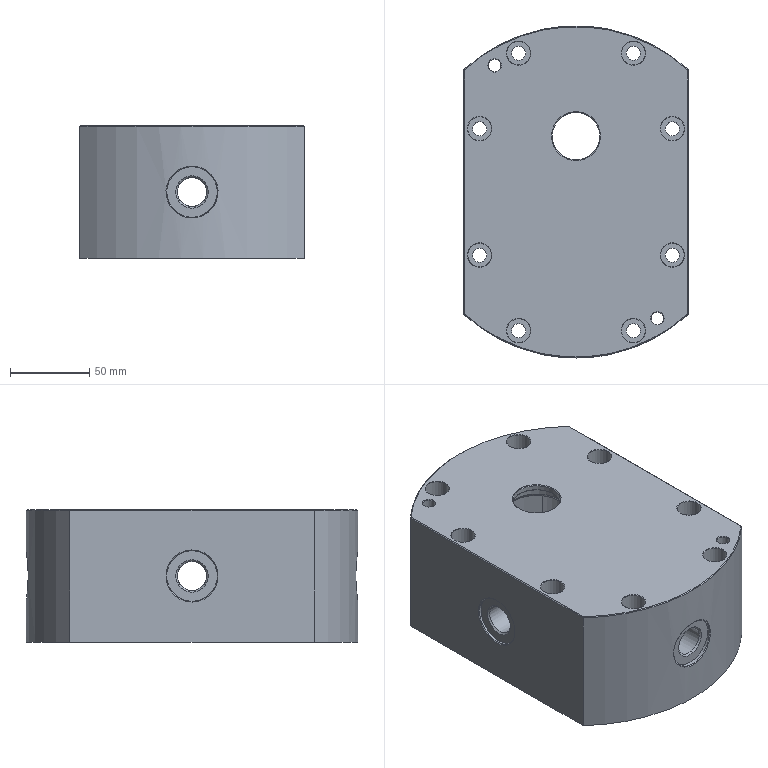NC program | NX | posted with a generic post | part box 142 x 210 x 84 mm
Whole program:
N10 G17 G21 G94 G90
(HOLE_MILLING_COPY_2 , TOOL : D10)
N12 T10 M6
N14 G54
N16 G17 G0 G90 X0. Y0. B0. C0. S3000 M3
N18 G43 Z30. H10
N20 Z0.634
N22 G94 G3 X-1.817 Y1.817 R1.817 F2200.
N24 X-3.633 Y0. R1.817
N26 X-3.633 Y0. Z0.414 I3.633 J0.
N28 X-3.633 Y0. Z0.194 I3.633 J0.
N30 X-3.633 Y0. Z-0.026 I3.633 J0.
N32 X-3.633 Y0. Z-0.246 I3.633 J0.
N34 X-3.633 Y0. Z-0.466 I3.633 J0.
N36 X-3.633 Y0. Z-0.686 I3.633 J0.
N38 X-3.633 Y0. Z-0.906 I3.633 J0.
N40 X-3.633 Y0. Z-1.126 I3.633 J0.
N42 X-3.633 Y0. Z-1.346 I3.633 J0.
N44 X-3.633 Y0. Z-1.566 I3.633 J0.
N46 X-3.633 Y0. Z-1.786 I3.633 J0.
N48 X-3.633 Y0. Z-2.006 I3.633 J0.
N50 X-3.633 Y0. Z-2.226 I3.633 J0.
N52 X-3.633 Y0. Z-2.446 I3.633 J0.
N54 X-3.633 Y0. Z-2.666 I3.633 J0.
N56 X-3.633 Y0. Z-2.886 I3.633 J0.
N58 X3.606 Y0.447 Z-3. R-3.633
N60 X-0.447 Y3.606 R3.633
N62 X3.606 Y0.447 R-3.633
N64 X1.58 Y2.026 R1.817
N66 X0. Y0. R1.817
N68 G0 Z0.634
N70 G3 X-3.633 Y3.633 R3.633
N72 X-7.267 Y0. R3.633
N74 X-7.267 Y0. Z0.414 I7.267 J0.
N76 X-7.267 Y0. Z0.194 I7.267 J0.
N78 X-7.267 Y0. Z-0.026 I7.267 J0.
N80 X-7.267 Y0. Z-0.246 I7.267 J0.
N82 X-7.267 Y0. Z-0.466 I7.267 J0.
N84 X-7.267 Y0. Z-0.686 I7.267 J0.
N86 X-7.267 Y0. Z-0.906 I7.267 J0.
N88 X-7.267 Y0. Z-1.126 I7.267 J0.
N90 X-7.267 Y0. Z-1.346 I7.267 J0.
N92 X-7.267 Y0. Z-1.566 I7.267 J0.
N94 X-7.267 Y0. Z-1.786 I7.267 J0.
N96 X-7.267 Y0. Z-2.006 I7.267 J0.
N98 X-7.267 Y0. Z-2.226 I7.267 J0.
N100 X-7.267 Y0. Z-2.446 I7.267 J0.
N102 X-7.267 Y0. Z-2.666 I7.267 J0.
N104 X-7.267 Y0. Z-2.886 I7.267 J0.
N106 X7.212 Y0.893 Z-3. R-7.267
N108 X-0.893 Y7.212 R7.267
N110 X7.212 Y0.893 R-7.267
N112 X3.159 Y4.052 R3.633
N114 X0. Y0. R3.633
N116 G0 Z0.634
N118 G3 X-5.45 Y5.45 R5.45
N120 X-10.9 Y0. R5.45
N122 X-10.9 Y0. Z0.414 I10.9 J0.
N124 X-10.9 Y0. Z0.194 I10.9 J0.
N126 X-10.9 Y0. Z-0.026 I10.9 J0.
N128 X-10.9 Y0. Z-0.246 I10.9 J0.
N130 X-10.9 Y0. Z-0.466 I10.9 J0.
N132 X-10.9 Y0. Z-0.686 I10.9 J0.
N134 X-10.9 Y0. Z-0.906 I10.9 J0.
N136 X-10.9 Y0. Z-1.126 I10.9 J0.
N138 X-10.9 Y0. Z-1.346 I10.9 J0.
N140 X-10.9 Y0. Z-1.566 I10.9 J0.
N142 X-10.9 Y0. Z-1.786 I10.9 J0.
N144 X-10.9 Y0. Z-2.006 I10.9 J0.
N146 X-10.9 Y0. Z-2.226 I10.9 J0.
N148 X-10.9 Y0. Z-2.446 I10.9 J0.
N150 X-10.9 Y0. Z-2.666 I10.9 J0.
N152 X-10.9 Y0. Z-2.886 I10.9 J0.
N154 X10.817 Y1.34 Z-3. R-10.9
N156 X-1.34 Y10.817 R10.9
N158 X10.817 Y1.34 R-10.9
N160 X4.739 Y6.079 R5.45
N162 X0. Y0. R5.45
N164 G0 Z30.
(HOLE_MILLING_COPY_COPY_1 , TOOL : D10)
N166 Z-2.5
N168 G3 X-2.075 Y2.075 R2.075
N170 X-4.15 Y0. R2.075
N172 X-4.15 Y0. Z-2.72 I4.15 J0.
N174 X-4.15 Y0. Z-2.94 I4.15 J0.
N176 X-4.15 Y0. Z-3.16 I4.15 J0.
N178 X-4.15 Y0. Z-3.38 I4.15 J0.
N180 X-4.15 Y0. Z-3.6 I4.15 J0.
N182 X-4.15 Y0. Z-3.82 I4.15 J0.
N184 X-4.15 Y0. Z-4.04 I4.15 J0.
N186 X-4.15 Y0. Z-4.26 I4.15 J0.
N188 X-4.15 Y0. Z-4.48 I4.15 J0.
N190 X-4.15 Y0. Z-4.7 I4.15 J0.
N192 X-4.15 Y0. Z-4.92 I4.15 J0.
N194 X-4.15 Y0. Z-5.14 I4.15 J0.
N196 X-4.15 Y0. Z-5.36 I4.15 J0.
N198 X-4.15 Y0. Z-5.58 I4.15 J0.
N200 X-4.15 Y0. Z-5.8 I4.15 J0.
N202 X-4.15 Y0. Z-6.02 I4.15 J0.
N204 X-4.15 Y0. Z-6.24 I4.15 J0.
N206 X-4.15 Y0. Z-6.46 I4.15 J0.
N208 X-4.15 Y0. Z-6.68 I4.15 J0.
N210 X-4.15 Y0. Z-6.9 I4.15 J0.
N212 X-4.15 Y0. Z-7.12 I4.15 J0.
N214 X-4.15 Y0. Z-7.34 I4.15 J0.
N216 X-4.15 Y0. Z-7.56 I4.15 J0.
N218 X-4.15 Y0. Z-7.78 I4.15 J0.
N220 X-4.15 Y0. Z-8. I4.15 J0.
N222 X-4.15 Y0. Z-8.22 I4.15 J0.
N224 X-4.15 Y0. Z-8.44 I4.15 J0.
N226 X-4.15 Y0. Z-8.66 I4.15 J0.
N228 X-4.15 Y0. Z-8.88 I4.15 J0.
N230 X-4.15 Y0. Z-9.1 I4.15 J0.
N232 X-4.15 Y0. Z-9.32 I4.15 J0.
N234 X-4.15 Y0. Z-9.54 I4.15 J0.
N236 X-4.15 Y0. Z-9.76 I4.15 J0.
N238 X-4.15 Y0. Z-9.98 I4.15 J0.
N240 X-4.15 Y0. Z-10.2 I4.15 J0.
N242 X-4.15 Y0. Z-10.42 I4.15 J0.
N244 X-4.15 Y0. Z-10.64 I4.15 J0.
N246 X-4.15 Y0. Z-10.86 I4.15 J0.
N248 X-4.15 Y0. Z-11.08 I4.15 J0.
N250 X-4.15 Y0. Z-11.3 I4.15 J0.
N252 X-4.15 Y0. Z-11.52 I4.15 J0.
N254 X-4.15 Y0. Z-11.74 I4.15 J0.
N256 X-4.15 Y0. Z-11.96 I4.15 J0.
N258 X-4.15 Y0. Z-12.18 I4.15 J0.
N260 X-4.15 Y0. Z-12.4 I4.15 J0.
N262 X-4.15 Y0. Z-12.62 I4.15 J0.
N264 X-4.15 Y0. Z-12.84 I4.15 J0.
N266 X-4.15 Y0. Z-13.06 I4.15 J0.
N268 X-4.15 Y0. Z-13.28 I4.15 J0.
N270 X-4.15 Y0. Z-13.5 I4.15 J0.
N272 X-4.15 Y0. Z-13.72 I4.15 J0.
N274 X-4.15 Y0. Z-13.94 I4.15 J0.
N276 X-4.15 Y0. Z-14.16 I4.15 J0.
N278 X-4.15 Y0. Z-14.38 I4.15 J0.
N280 X-4.15 Y0. Z-14.6 I4.15 J0.
N282 X-4.15 Y0. Z-14.82 I4.15 J0.
N284 X-4.15 Y0. Z-15.04 I4.15 J0.
N286 X-4.15 Y0. Z-15.26 I4.15 J0.
N288 X-4.15 Y0. Z-15.48 I4.15 J0.
N290 X-4.15 Y0. Z-15.7 I4.15 J0.
N292 X-4.15 Y0. Z-15.92 I4.15 J0.
N294 X-4.15 Y0. Z-16.14 I4.15 J0.
N296 X-4.15 Y0. Z-16.36 I4.15 J0.
N298 X-4.15 Y0. Z-16.58 I4.15 J0.
N300 X-4.15 Y0. Z-16.8 I4.15 J0.
N302 X-4.15 Y0. Z-17.02 I4.15 J0.
N304 X-4.15 Y0. Z-17.24 I4.15 J0.
N306 X-4.15 Y0. Z-17.46 I4.15 J0.
N308 X-4.15 Y0. Z-17.68 I4.15 J0.
N310 X-4.15 Y0. Z-17.9 I4.15 J0.
N312 X-4.15 Y0. Z-18.12 I4.15 J0.
N314 X-4.15 Y0. Z-18.34 I4.15 J0.
N316 X-4.15 Y0. Z-18.56 I4.15 J0.
N318 X-4.15 Y0. Z-18.78 I4.15 J0.
N320 X-4.15 Y0. Z-19. I4.15 J0.
N322 X-4.15 Y0. Z-19.22 I4.15 J0.
N324 X-4.15 Y0. Z-19.44 I4.15 J0.
N326 X-4.15 Y0. Z-19.66 I4.15 J0.
N328 X-4.15 Y0. Z-19.88 I4.15 J0.
N330 X-4.15 Y0. Z-20.1 I4.15 J0.
N332 X-4.15 Y0. Z-20.32 I4.15 J0.
N334 X-4.15 Y0. Z-20.54 I4.15 J0.
N336 X-4.15 Y0. Z-20.76 I4.15 J0.
N338 X-4.15 Y0. Z-20.98 I4.15 J0.
N340 X-4.15 Y0. Z-21.2 I4.15 J0.
N342 X-4.15 Y0. Z-21.42 I4.15 J0.
N344 X-4.15 Y0. Z-21.64 I4.15 J0.
N346 X-4.15 Y0. Z-21.86 I4.15 J0.
N348 X-4.15 Y0. Z-22.08 I4.15 J0.
N350 X-4.15 Y0. Z-22.3 I4.15 J0.
N352 X-4.15 Y0. Z-22.52 I4.15 J0.
N354 X-4.15 Y0. Z-22.74 I4.15 J0.
N356 X-4.15 Y0. Z-22.96 I4.15 J0.
N358 X-4.15 Y0. Z-23.18 I4.15 J0.
N360 X-4.15 Y0. Z-23.4 I4.15 J0.
N362 X-4.15 Y0. Z-23.62 I4.15 J0.
N364 X-4.15 Y0. Z-23.84 I4.15 J0.
N366 X0.591 Y4.108 Z-24. R-4.15
N368 X-4.108 Y0.591 R4.15
N370 X0.591 Y4.108 R-4.15
N372 X-1.759 Y2.349 R2.075
N374 X0. Y0. R2.075
N376 G0 Z30.
N378 M5
(HOLE_MILLING_COPY_1_COPY_2 , TOOL : D10JING)
N380 T11 M6
N382 G54
N384 G17 G0 G90 X0. Y0. B0. C0. S5000 M3
N386 G43 Z30. H11
N388 Z-3.
N390 G94 G1 X-7.486 Y2.524 F1000.
N392 G3 X-11. Y0. R2.663
N394 X0. Y-11. R11.
N396 X-11. Y0. R-11.
N398 X-7.486 Y-2.524 R2.663
N400 G1 X0. Y0.
N402 G0 Z30.
(HOLE_MILLING_COPY_1_COPY_COPY , TOOL : D10JING)
N404 Z-24.
N406 G1 X-0.58 Y0.993
N408 G3 X-4.25 Y0. R1.969
N410 X0. Y-4.25 R4.25
N412 X-4.25 Y0. R-4.25
N414 X-0.58 Y-0.993 R1.969
N416 G1 X0. Y0.
N418 G0 Z30.
N420 M5
(PLANAR_MILL_COPY_COPY_COPY_1 , TOOL : D6A45)
N422 T07 M6
N424 G54
N426 G17 G0 G90 X1.621 Y7.374 B0. C0. S7500 M3
N428 G43 Z30. H7
N430 Z-1.5
N432 G94 G1 Z-4.5 F1250.
N434 X0.766 Y8.393
N436 G3 X0. Y8.75 R1.
N438 X-8.75 Y0. R8.75
N440 X0. Y8.75 R-8.75
N442 X-0.766 Y8.393 R1.
N444 G1 X-1.621 Y7.374
N446 Z-1.5
N448 G0 Z30.
(PROFILE_3D , TOOL : D6A45)
N450 X-1.069 Y-14.174
N452 Z1.978
N454 G1 Z-1.022
N456 X-0.407 Y-15.166
N458 G3 X0.131 Y-15.432 R0.6
N460 G1 X1.879 Y-15.319 Z-1.02
N462 X3.594 Y-15.012 Z-1.093
N464 X5.177 Y-14.547 Z-1.163
N466 X6.702 Y-13.916 Z-1.232
N468 X8.15 Y-13.128 Z-1.364
N470 X9.505 Y-12.192 Z-1.496
N472 X10.752 Y-11.118 Z-1.628
N474 X11.876 Y-9.917 Z-1.759
N476 X12.867 Y-8.602 Z-1.891
N478 X13.711 Y-7.188 Z-2.023
N480 X14.401 Y-5.691 Z-2.103
N482 X14.926 Y-4.129 Z-2.182
N484 X15.297 Y-2.432 Z-2.267
N486 X15.473 Y-0.704 Z-2.278
N488 X15.454 Y1.033 Z-2.289
N490 X15.239 Y2.756 Z-2.224
N492 X14.832 Y4.444 Z-2.159
N494 X14.238 Y6.075 Z-2.095
N496 X13.466 Y7.628 Z-1.966
N498 X12.524 Y9.082 Z-1.837
N500 X11.366 Y10.486 Z-1.702
N502 X10.052 Y11.744 Z-1.567
N504 X8.6 Y12.839 Z-1.431
N506 X7.028 Y13.756 Z-1.296
N508 X5.36 Y14.482 Z-1.161
N510 X3.616 Y15.009 Z-1.089
N512 X1.821 Y15.327 Z-1.017
N514 X-0.006 Y15.434 Z-1.028
N516 X-1.476 Y15.365 Z-1.037
N518 X-2.937 Y15.155 Z-1.045
N520 X-4.372 Y14.807 Z-1.12
N522 X-5.767 Y14.325 Z-1.195
N524 X-7.109 Y13.713 Z-1.27
N526 X-8.38 Y12.98 Z-1.384
N528 X-9.873 Y11.892 Z-1.527
N530 X-11.222 Y10.639 Z-1.669
N532 X-12.412 Y9.234 Z-1.812
N534 X-13.427 Y7.698 Z-1.955
N536 X-14.251 Y6.053 Z-2.097
N538 X-14.873 Y4.319 Z-2.182
N540 X-15.283 Y2.522 Z-2.266
N542 X-15.476 Y0.688 Z-2.3
N544 X-15.449 Y-1.147 Z-2.278
N546 X-15.204 Y-2.966 Z-2.257
N548 X-14.744 Y-4.741 Z-2.163
N550 X-14.076 Y-6.447 Z-2.07
N552 X-13.21 Y-8.062 Z-1.93
N554 X-12.159 Y-9.563 Z-1.791
N556 X-10.938 Y-10.929 Z-1.652
N558 X-9.563 Y-12.142 Z-1.513
N560 X-8.138 Y-13.132 Z-1.382
N562 X-6.608 Y-13.958 Z-1.25
N564 X-4.994 Y-14.608 Z-1.174
N566 X-3.317 Y-15.074 Z-1.099
N568 X-1.598 Y-15.35 Z-1.023
N570 X0.131 Y-15.432 Z-1.022
N572 G3 X0.665 Y-15.157 R0.6
N574 G1 X1.308 Y-14.154
N576 Z1.978
N578 G0 Z30.
N580 M5
N582 M2